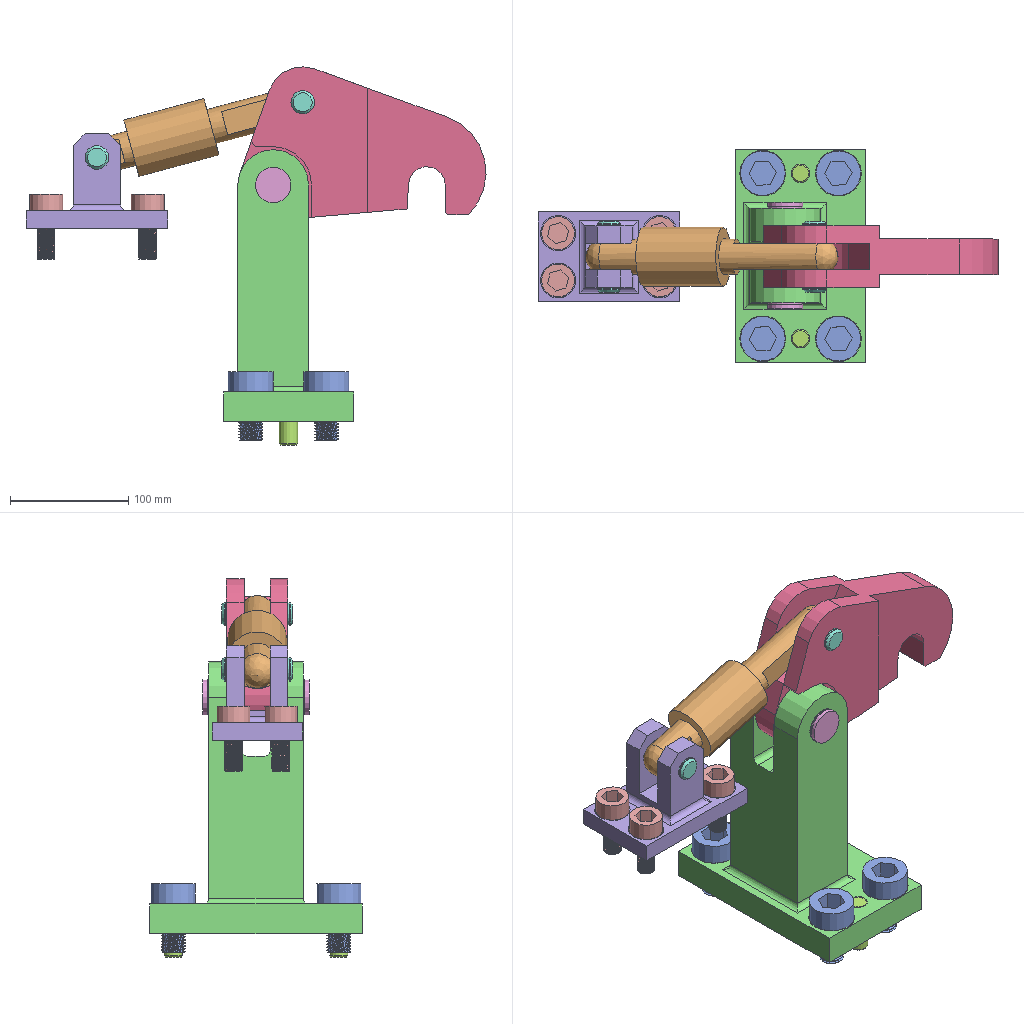Assembly | NX | 9 different items | 17 placed | box 389 x 180 x 320 mm
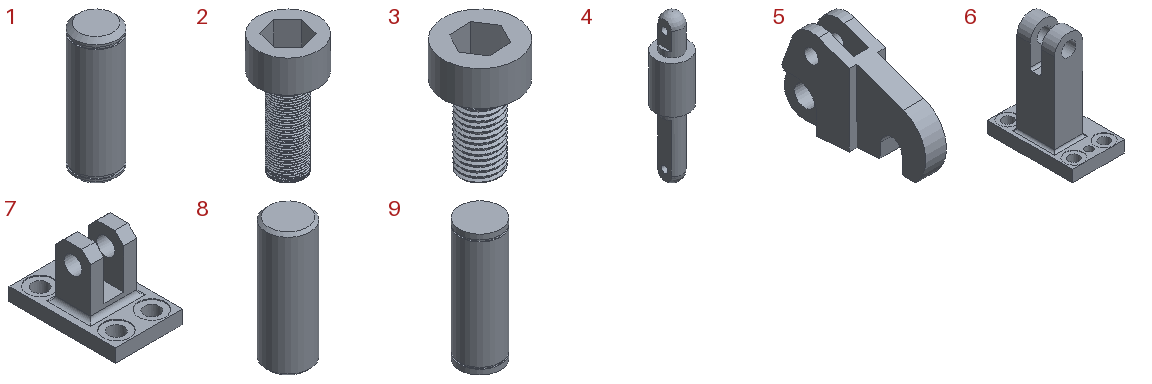Parts list (item | quantity | size | volume | features):
1 | x2 | 20 x 20 x 60 mm | 18548 mm3 | features DATUM_CSYS 2, CHAMFER 1, SKETCH 1, SWP104 1
2 | x4 | 28 x 28 x 55 mm | 12823 mm3 | features DATUM_CSYS 4, EXTRUDE 3, SKETCH 3, THREADS 1
3 | x4 | 38 x 38 x 58 mm | 26254 mm3 | features DATUM_CSYS 4, EXTRUDE 3, SKETCH 3, SYMBOLIC_THREAD 1, THREADS 1
4 | x1 | 50 x 50 x 220 mm | 220357 mm3 | features DATUM_CSYS 6, EXTRUDE 5, SKETCH 5, BLEND 2
5 | x1 | 52 x 210 x 130 mm | 615781 mm3 | features DATUM_CSYS 7, EXTRUDE 6, SKETCH 6, EXTRACT_FACE 2, CHAMFER 1, Instance Feature 1, Mirror Feature 1
6 | x1 | 110 x 180 x 230 mm | 1253704 mm3 | features DATUM_CSYS 6, SKETCH 5, CBORE_HOLE 4, EXTRUDE 3, HOLE PACKAGE 3, SIMPLE HOLE 3, BLEND 2
7 | x1 | 76 x 120 x 80 mm | 195913 mm3 | features DATUM_CSYS 6, EXTRUDE 5, SKETCH 5, BLEND 1, CHAMFER 1
8 | x2 | 15.8 x 15.8 x 45 mm | 8775 mm3 | features DATUM_CSYS 2, CHAMFER 1, EXTRUDE 1, SKETCH 1
9 | x1 | 30 x 30 x 90 mm | 63450 mm3 | features DATUM_CSYS 2, SKETCH 1, SWP104 1
Mates (type | each side: item.copy, entity, surface, feature):
Concentric | 5.1 edge | 6.1 edge
Concentric | 4.1 edge | 5.1 edge
Touch | 7.1 face plane Extrude(3) | 4.1 face plane Extrude(4)
Concentric | 7.1 edge | 4.1 edge
Concentric | 1.1 edge | 7.1 edge
Concentric | 9.1 edge | 6.1 edge
Concentric | 1.1 edge | 5.1 edge
Concentric | 8.1 edge | 6.1 edge
Concentric | 3.1 edge | 6.1 edge
Concentric | 2.1 edge | 7.1 edge